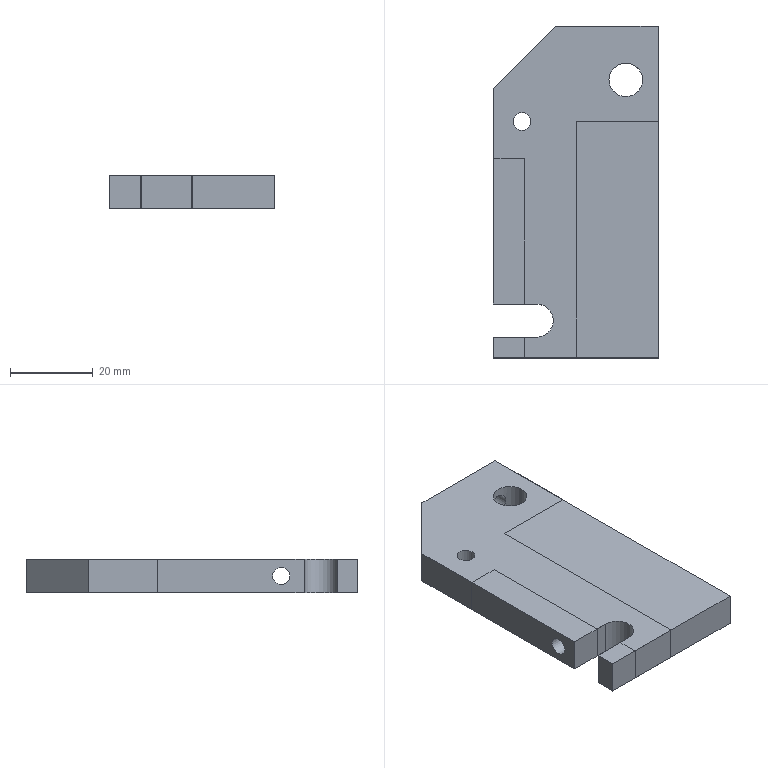Part | 2 solids | 42 faces | box 40 x 80 x 8 mm | volume 34060 mm3 | plane 32 | cylinder 10 | commonest cylinder face diameters 4.2 x4 4.3 x2 8 x2 8.1 x2
STEP:
#1=CARTESIAN_POINT('',(20.,39.8,-8.));
#2=VERTEX_POINT('',#1);
#3=CARTESIAN_POINT('',(19.8,40.,-8.));
#4=VERTEX_POINT('',#3);
#5=CARTESIAN_POINT('',(20.,39.8,-8.));
#6=DIRECTION('',(-0.7071,0.7071,0.));
#7=VECTOR('',#6,1000.);
#8=LINE('',#5,#7);
#9=EDGE_CURVE('',#2,#4,#8,.T.);
#10=ORIENTED_EDGE('',*,*,#9,.T.);
#11=CARTESIAN_POINT('',(19.8,40.,0.));
#12=VERTEX_POINT('',#11);
#13=CARTESIAN_POINT('',(19.8,40.,-8.));
#14=DIRECTION('',(0.,0.,-1.));
#15=VECTOR('',#14,1000.);
#16=LINE('',#13,#15);
#17=EDGE_CURVE('',#12,#4,#16,.T.);
#18=ORIENTED_EDGE('',*,*,#17,.F.);
#19=CARTESIAN_POINT('',(20.,39.8,0.));
#20=VERTEX_POINT('',#19);
#21=CARTESIAN_POINT('',(40.65,19.15,0.));
#22=DIRECTION('',(0.7071,-0.7071,0.));
#23=VECTOR('',#22,1000.);
#24=LINE('',#21,#23);
#25=EDGE_CURVE('',#12,#20,#24,.T.);
#26=ORIENTED_EDGE('',*,*,#25,.T.);
#27=CARTESIAN_POINT('',(20.,39.8,-8.));
#28=DIRECTION('',(0.,0.,1.));
#29=VECTOR('',#28,1000.);
#30=LINE('',#27,#29);
#31=EDGE_CURVE('',#2,#20,#30,.T.);
#32=ORIENTED_EDGE('',*,*,#31,.F.);
#33=EDGE_LOOP('',(#10,#18,#26,#32));
#34=FACE_BOUND('',#33,.T.);
#35=CARTESIAN_POINT('',(20.,39.8,-8.));
#36=DIRECTION('',(-0.7071,-0.7071,0.));
#37=DIRECTION('',(0.,0.,1.));
#38=AXIS2_PLACEMENT_3D('',#35,#36,#37);
#39=PLANE('',#38);
#40=ADVANCED_FACE('',(#34),#39,.F.);
#41=CARTESIAN_POINT('',(-20.,-21.5,-6.1));
#42=VERTEX_POINT('',#41);
#43=CARTESIAN_POINT('',(-20.,-21.5,-4.));
#44=DIRECTION('',(1.,0.,0.));
#45=DIRECTION('',(0.,0.,-1.));
#46=AXIS2_PLACEMENT_3D('',#43,#44,#45);
#47=CIRCLE('',#46,2.1);
#48=EDGE_CURVE('',#42,#42,#47,.F.);
#49=ORIENTED_EDGE('',*,*,#48,.T.);
#50=EDGE_LOOP('',(#49));
#51=FACE_BOUND('',#50,.T.);
#52=CARTESIAN_POINT('',(20.,-21.5,-1.9));
#53=VERTEX_POINT('',#52);
#54=CARTESIAN_POINT('',(20.,-21.5,-4.));
#55=DIRECTION('',(-1.,0.,0.));
#56=DIRECTION('',(0.,0.,1.));
#57=AXIS2_PLACEMENT_3D('',#54,#55,#56);
#58=CIRCLE('',#57,2.1);
#59=EDGE_CURVE('',#53,#53,#58,.F.);
#60=ORIENTED_EDGE('',*,*,#59,.T.);
#61=EDGE_LOOP('',(#60));
#62=FACE_BOUND('',#61,.T.);
#63=CARTESIAN_POINT('',(0.1,-21.5,-4.));
#64=DIRECTION('',(-1.,0.,0.));
#65=DIRECTION('',(0.,0.,1.));
#66=AXIS2_PLACEMENT_3D('',#63,#64,#65);
#67=CYLINDRICAL_SURFACE('',#66,2.1);
#68=ADVANCED_FACE('',(#51,#62),#67,.F.);
#69=CARTESIAN_POINT('',(12.,31.05,-1.9));
#70=VERTEX_POINT('',#69);
#71=CARTESIAN_POINT('',(12.704,31.005,-1.982));
#72=CARTESIAN_POINT('',(12.022,31.078,-1.85));
#73=CARTESIAN_POINT('',(11.33,31.011,-1.971));
#74=CARTESIAN_POINT('',(10.827,30.881,-2.248));
#75=CARTESIAN_POINT('',(10.609,30.808,-2.406));
#76=CARTESIAN_POINT('',(10.332,30.692,-2.717));
#77=CARTESIAN_POINT('',(10.245,30.65,-2.843));
#78=CARTESIAN_POINT('',(10.049,30.552,-3.178));
#79=CARTESIAN_POINT('',(9.934,30.483,-3.561));
#80=CARTESIAN_POINT('',(9.886,30.454,-3.986));
#81=CARTESIAN_POINT('',(9.923,30.477,-4.399));
#82=CARTESIAN_POINT('',(10.032,30.54,-4.747));
#83=CARTESIAN_POINT('',(10.127,30.592,-4.96));
#84=CARTESIAN_POINT('',(10.26,30.657,-5.18));
#85=CARTESIAN_POINT('',(10.309,30.681,-5.25));
#86=CARTESIAN_POINT('',(10.494,30.762,-5.473));
#87=CARTESIAN_POINT('',(10.676,30.828,-5.633));
#88=CARTESIAN_POINT('',(10.855,30.887,-5.768));
#89=CARTESIAN_POINT('',(11.288,31.003,-6.012));
#90=CARTESIAN_POINT('',(11.973,31.078,-6.15));
#91=CARTESIAN_POINT('',(12.659,31.013,-6.034));
#92=CARTESIAN_POINT('',(13.172,30.881,-5.752));
#93=CARTESIAN_POINT('',(13.393,30.807,-5.592));
#94=CARTESIAN_POINT('',(13.668,30.692,-5.283));
#95=CARTESIAN_POINT('',(13.756,30.65,-5.156));
#96=CARTESIAN_POINT('',(13.95,30.552,-4.823));
#97=CARTESIAN_POINT('',(14.067,30.483,-4.439));
#98=CARTESIAN_POINT('',(14.114,30.455,-4.013));
#99=CARTESIAN_POINT('',(14.078,30.477,-3.605));
#100=CARTESIAN_POINT('',(13.969,30.54,-3.254));
#101=CARTESIAN_POINT('',(13.873,30.592,-3.042));
#102=CARTESIAN_POINT('',(13.743,30.656,-2.824));
#103=CARTESIAN_POINT('',(13.691,30.681,-2.751));
#104=CARTESIAN_POINT('',(13.508,30.761,-2.529));
#105=CARTESIAN_POINT('',(13.326,30.828,-2.369));
#106=CARTESIAN_POINT('',(13.148,30.886,-2.235));
#107=CARTESIAN_POINT('',(12.704,31.005,-1.982));
#108=CARTESIAN_POINT('',(12.022,31.078,-1.85));
#109=CARTESIAN_POINT('',(11.33,31.011,-1.971));
#110=B_SPLINE_CURVE_WITH_KNOTS('',3,(#71,#72,#73,#74,#75,#76,#77,#78,#79,#80,#81,#82,#83,#84,#85,#86,#87,#88,#89,#90,#91,#92,#93,#94,#95,#96,#97,#98,#99,#100,#101,#102,#103,#104,#105,#106,#107,#108,#109),.UNSPECIFIED.,.T.,.F.,(1,1,1,1,1,1,1,1,1,1,1,1,1,1,1,1,1,1,1,1,1,1,1,1,1,1,1,1,1,1,1,1,1,1,1,1,1,1,1,1,1,1,1),(-0.111,-0.09539,-0.06414,0.,0.05937,0.09203,0.1234,0.139,0.1546,0.1859,0.2171,0.2484,0.2796,0.3109,0.3265,0.3421,0.3577,0.3734,0.389,0.4046,0.4359,0.4968,0.5592,0.592,0.6234,0.639,0.6546,0.6859,0.7171,0.7484,0.7796,0.8109,0.8265,0.8421,0.8577,0.8734,0.889,0.9046,0.9359,1.,1.059,1.092,1.123),.UNSPECIFIED.);
#111=EDGE_CURVE('',#70,#70,#110,.F.);
#112=ORIENTED_EDGE('',*,*,#111,.F.);
#113=EDGE_LOOP('',(#112));
#114=FACE_BOUND('',#113,.T.);
#115=CARTESIAN_POINT('',(9.9,40.,-4.));
#116=VERTEX_POINT('',#115);
#117=CARTESIAN_POINT('',(12.,40.,-4.));
#118=DIRECTION('',(0.,1.,0.));
#119=DIRECTION('',(-1.,0.,0.));
#120=AXIS2_PLACEMENT_3D('',#117,#118,#119);
#121=CIRCLE('',#120,2.1);
#122=EDGE_CURVE('',#116,#116,#121,.T.);
#123=ORIENTED_EDGE('',*,*,#122,.T.);
#124=EDGE_LOOP('',(#123));
#125=FACE_BOUND('',#124,.T.);
#126=CARTESIAN_POINT('',(12.,27.,-4.));
#127=DIRECTION('',(0.,1.,0.));
#128=DIRECTION('',(0.,0.,1.));
#129=AXIS2_PLACEMENT_3D('',#126,#127,#128);
#130=CYLINDRICAL_SURFACE('',#129,2.1);
#131=ADVANCED_FACE('',(#114,#125),#130,.F.);
#132=CARTESIAN_POINT('',(16.05,27.,0.));
#133=VERTEX_POINT('',#132);
#134=CARTESIAN_POINT('',(12.,27.,0.));
#135=DIRECTION('',(0.,0.,1.));
#136=DIRECTION('',(1.,0.,0.));
#137=AXIS2_PLACEMENT_3D('',#134,#135,#136);
#138=CIRCLE('',#137,4.05);
#139=EDGE_CURVE('',#133,#133,#138,.T.);
#140=ORIENTED_EDGE('',*,*,#139,.F.);
#141=EDGE_LOOP('',(#140));
#142=FACE_BOUND('',#141,.T.);
#143=CARTESIAN_POINT('',(-10.85,17.,0.));
#144=VERTEX_POINT('',#143);
#145=CARTESIAN_POINT('',(-13.,17.,0.));
#146=DIRECTION('',(0.,0.,1.));
#147=DIRECTION('',(1.,0.,0.));
#148=AXIS2_PLACEMENT_3D('',#145,#146,#147);
#149=CIRCLE('',#148,2.15);
#150=EDGE_CURVE('',#144,#144,#149,.T.);
#151=ORIENTED_EDGE('',*,*,#150,.F.);
#152=EDGE_LOOP('',(#151));
#153=FACE_BOUND('',#152,.T.);
#154=CARTESIAN_POINT('',(-9.5,-35.,0.));
#155=VERTEX_POINT('',#154);
#156=CARTESIAN_POINT('',(-20.,-35.,0.));
#157=VERTEX_POINT('',#156);
#158=CARTESIAN_POINT('',(-9.5,-35.,0.));
#159=DIRECTION('',(-1.,0.,0.));
#160=VECTOR('',#159,1000.);
#161=LINE('',#158,#160);
#162=EDGE_CURVE('',#155,#157,#161,.T.);
#163=ORIENTED_EDGE('',*,*,#162,.T.);
#164=CARTESIAN_POINT('',(-20.,-40.,0.));
#165=VERTEX_POINT('',#164);
#166=CARTESIAN_POINT('',(-20.,-31.,0.));
#167=DIRECTION('',(0.,1.,0.));
#168=VECTOR('',#167,1000.);
#169=LINE('',#166,#168);
#170=EDGE_CURVE('',#165,#157,#169,.T.);
#171=ORIENTED_EDGE('',*,*,#170,.F.);
#172=CARTESIAN_POINT('',(20.,-40.,0.));
#173=VERTEX_POINT('',#172);
#174=CARTESIAN_POINT('',(0.,-40.,0.));
#175=DIRECTION('',(-1.,0.,0.));
#176=VECTOR('',#175,1000.);
#177=LINE('',#174,#176);
#178=EDGE_CURVE('',#173,#165,#177,.T.);
#179=ORIENTED_EDGE('',*,*,#178,.F.);
#180=CARTESIAN_POINT('',(20.,40.,0.));
#181=DIRECTION('',(0.,-1.,0.));
#182=VECTOR('',#181,1000.);
#183=LINE('',#180,#182);
#184=EDGE_CURVE('',#173,#20,#183,.F.);
#185=ORIENTED_EDGE('',*,*,#184,.T.);
#186=ORIENTED_EDGE('',*,*,#25,.F.);
#187=CARTESIAN_POINT('',(-5.,40.,0.));
#188=VERTEX_POINT('',#187);
#189=CARTESIAN_POINT('',(-5.,40.,0.));
#190=DIRECTION('',(1.,0.,0.));
#191=VECTOR('',#190,1000.);
#192=LINE('',#189,#191);
#193=EDGE_CURVE('',#188,#12,#192,.T.);
#194=ORIENTED_EDGE('',*,*,#193,.F.);
#195=CARTESIAN_POINT('',(-20.,25.,0.));
#196=VERTEX_POINT('',#195);
#197=CARTESIAN_POINT('',(-20.,25.,0.));
#198=DIRECTION('',(0.7071,0.7071,0.));
#199=VECTOR('',#198,1000.);
#200=LINE('',#197,#199);
#201=EDGE_CURVE('',#196,#188,#200,.T.);
#202=ORIENTED_EDGE('',*,*,#201,.F.);
#203=CARTESIAN_POINT('',(-20.,-27.,0.));
#204=VERTEX_POINT('',#203);
#205=CARTESIAN_POINT('',(-20.,-31.,0.));
#206=DIRECTION('',(0.,1.,0.));
#207=VECTOR('',#206,1000.);
#208=LINE('',#205,#207);
#209=EDGE_CURVE('',#204,#196,#208,.T.);
#210=ORIENTED_EDGE('',*,*,#209,.F.);
#211=CARTESIAN_POINT('',(-9.5,-27.,0.));
#212=VERTEX_POINT('',#211);
#213=CARTESIAN_POINT('',(-9.5,-27.,0.));
#214=DIRECTION('',(-1.,0.,0.));
#215=VECTOR('',#214,1000.);
#216=LINE('',#213,#215);
#217=EDGE_CURVE('',#212,#204,#216,.T.);
#218=ORIENTED_EDGE('',*,*,#217,.F.);
#219=CARTESIAN_POINT('',(-9.5,-31.,0.));
#220=DIRECTION('',(0.,0.,1.));
#221=DIRECTION('',(1.,0.,0.));
#222=AXIS2_PLACEMENT_3D('',#219,#220,#221);
#223=CIRCLE('',#222,4.);
#224=EDGE_CURVE('',#155,#212,#223,.T.);
#225=ORIENTED_EDGE('',*,*,#224,.F.);
#226=EDGE_LOOP('',(#163,#171,#179,#185,#186,#194,#202,#210,#218,#225));
#227=FACE_BOUND('',#226,.T.);
#228=CARTESIAN_POINT('',(-9.5,-31.,0.));
#229=DIRECTION('',(0.,0.,1.));
#230=DIRECTION('',(1.,0.,0.));
#231=AXIS2_PLACEMENT_3D('',#228,#229,#230);
#232=PLANE('',#231);
#233=ADVANCED_FACE('',(#142,#153,#227),#232,.T.);
#234=CARTESIAN_POINT('',(16.05,27.,-8.));
#235=VERTEX_POINT('',#234);
#236=CARTESIAN_POINT('',(12.,27.,-8.));
#237=DIRECTION('',(0.,0.,1.));
#238=DIRECTION('',(1.,0.,0.));
#239=AXIS2_PLACEMENT_3D('',#236,#237,#238);
#240=CIRCLE('',#239,4.05);
#241=EDGE_CURVE('',#235,#235,#240,.T.);
#242=ORIENTED_EDGE('',*,*,#241,.T.);
#243=EDGE_LOOP('',(#242));
#244=FACE_BOUND('',#243,.T.);
#245=CARTESIAN_POINT('',(-10.85,17.,-8.));
#246=VERTEX_POINT('',#245);
#247=CARTESIAN_POINT('',(-13.,17.,-8.));
#248=DIRECTION('',(0.,0.,1.));
#249=DIRECTION('',(1.,0.,0.));
#250=AXIS2_PLACEMENT_3D('',#247,#248,#249);
#251=CIRCLE('',#250,2.15);
#252=EDGE_CURVE('',#246,#246,#251,.T.);
#253=ORIENTED_EDGE('',*,*,#252,.T.);
#254=EDGE_LOOP('',(#253));
#255=FACE_BOUND('',#254,.T.);
#256=CARTESIAN_POINT('',(-20.,-40.,-8.));
#257=VERTEX_POINT('',#256);
#258=CARTESIAN_POINT('',(-20.,-35.,-8.));
#259=VERTEX_POINT('',#258);
#260=CARTESIAN_POINT('',(-20.,-31.,-8.));
#261=DIRECTION('',(0.,1.,0.));
#262=VECTOR('',#261,1000.);
#263=LINE('',#260,#262);
#264=EDGE_CURVE('',#257,#259,#263,.T.);
#265=ORIENTED_EDGE('',*,*,#264,.T.);
#266=CARTESIAN_POINT('',(-9.5,-35.,-8.));
#267=VERTEX_POINT('',#266);
#268=CARTESIAN_POINT('',(-9.5,-35.,-8.));
#269=DIRECTION('',(-1.,0.,0.));
#270=VECTOR('',#269,1000.);
#271=LINE('',#268,#270);
#272=EDGE_CURVE('',#267,#259,#271,.T.);
#273=ORIENTED_EDGE('',*,*,#272,.F.);
#274=CARTESIAN_POINT('',(-9.5,-27.,-8.));
#275=VERTEX_POINT('',#274);
#276=CARTESIAN_POINT('',(-9.5,-31.,-8.));
#277=DIRECTION('',(0.,0.,1.));
#278=DIRECTION('',(1.,0.,0.));
#279=AXIS2_PLACEMENT_3D('',#276,#277,#278);
#280=CIRCLE('',#279,4.);
#281=EDGE_CURVE('',#267,#275,#280,.T.);
#282=ORIENTED_EDGE('',*,*,#281,.T.);
#283=CARTESIAN_POINT('',(-20.,-27.,-8.));
#284=VERTEX_POINT('',#283);
#285=CARTESIAN_POINT('',(-9.5,-27.,-8.));
#286=DIRECTION('',(-1.,0.,0.));
#287=VECTOR('',#286,1000.);
#288=LINE('',#285,#287);
#289=EDGE_CURVE('',#275,#284,#288,.T.);
#290=ORIENTED_EDGE('',*,*,#289,.T.);
#291=CARTESIAN_POINT('',(-20.,25.,-8.));
#292=VERTEX_POINT('',#291);
#293=CARTESIAN_POINT('',(-20.,-31.,-8.));
#294=DIRECTION('',(0.,1.,0.));
#295=VECTOR('',#294,1000.);
#296=LINE('',#293,#295);
#297=EDGE_CURVE('',#284,#292,#296,.T.);
#298=ORIENTED_EDGE('',*,*,#297,.T.);
#299=CARTESIAN_POINT('',(-5.,40.,-8.));
#300=VERTEX_POINT('',#299);
#301=CARTESIAN_POINT('',(-20.,25.,-8.));
#302=DIRECTION('',(0.7071,0.7071,0.));
#303=VECTOR('',#302,1000.);
#304=LINE('',#301,#303);
#305=EDGE_CURVE('',#292,#300,#304,.T.);
#306=ORIENTED_EDGE('',*,*,#305,.T.);
#307=CARTESIAN_POINT('',(-5.,40.,-8.));
#308=DIRECTION('',(1.,0.,0.));
#309=VECTOR('',#308,1000.);
#310=LINE('',#307,#309);
#311=EDGE_CURVE('',#300,#4,#310,.T.);
#312=ORIENTED_EDGE('',*,*,#311,.T.);
#313=ORIENTED_EDGE('',*,*,#9,.F.);
#314=CARTESIAN_POINT('',(20.,-40.,-8.));
#315=VERTEX_POINT('',#314);
#316=CARTESIAN_POINT('',(20.,40.,-8.));
#317=DIRECTION('',(0.,-1.,0.));
#318=VECTOR('',#317,1000.);
#319=LINE('',#316,#318);
#320=EDGE_CURVE('',#315,#2,#319,.F.);
#321=ORIENTED_EDGE('',*,*,#320,.F.);
#322=CARTESIAN_POINT('',(0.,-40.,-8.));
#323=DIRECTION('',(-1.,0.,0.));
#324=VECTOR('',#323,1000.);
#325=LINE('',#322,#324);
#326=EDGE_CURVE('',#315,#257,#325,.T.);
#327=ORIENTED_EDGE('',*,*,#326,.T.);
#328=EDGE_LOOP('',(#265,#273,#282,#290,#298,#306,#312,#313,#321,#327));
#329=FACE_BOUND('',#328,.T.);
#330=CARTESIAN_POINT('',(-9.5,-31.,-8.));
#331=DIRECTION('',(0.,0.,1.));
#332=DIRECTION('',(1.,0.,0.));
#333=AXIS2_PLACEMENT_3D('',#330,#331,#332);
#334=PLANE('',#333);
#335=ADVANCED_FACE('',(#244,#255,#329),#334,.F.);
#336=ORIENTED_EDGE('',*,*,#150,.T.);
#337=EDGE_LOOP('',(#336));
#338=FACE_BOUND('',#337,.T.);
#339=ORIENTED_EDGE('',*,*,#252,.F.);
#340=EDGE_LOOP('',(#339));
#341=FACE_BOUND('',#340,.T.);
#342=CARTESIAN_POINT('',(-13.,17.,-8.));
#343=DIRECTION('',(0.,0.,1.));
#344=DIRECTION('',(1.,0.,0.));
#345=AXIS2_PLACEMENT_3D('',#342,#343,#344);
#346=CYLINDRICAL_SURFACE('',#345,2.15);
#347=ADVANCED_FACE('',(#338,#341),#346,.F.);
#348=ORIENTED_EDGE('',*,*,#111,.T.);
#349=EDGE_LOOP('',(#348));
#350=FACE_BOUND('',#349,.T.);
#351=ORIENTED_EDGE('',*,*,#139,.T.);
#352=EDGE_LOOP('',(#351));
#353=FACE_BOUND('',#352,.T.);
#354=ORIENTED_EDGE('',*,*,#241,.F.);
#355=EDGE_LOOP('',(#354));
#356=FACE_BOUND('',#355,.T.);
#357=CARTESIAN_POINT('',(12.,27.,-8.));
#358=DIRECTION('',(0.,0.,1.));
#359=DIRECTION('',(1.,0.,0.));
#360=AXIS2_PLACEMENT_3D('',#357,#358,#359);
#361=CYLINDRICAL_SURFACE('',#360,4.05);
#362=ADVANCED_FACE('',(#350,#353,#356),#361,.F.);
#363=ORIENTED_EDGE('',*,*,#320,.T.);
#364=ORIENTED_EDGE('',*,*,#31,.T.);
#365=ORIENTED_EDGE('',*,*,#184,.F.);
#366=CARTESIAN_POINT('',(20.,-40.,-8.));
#367=DIRECTION('',(0.,0.,1.));
#368=VECTOR('',#367,1000.);
#369=LINE('',#366,#368);
#370=EDGE_CURVE('',#173,#315,#369,.F.);
#371=ORIENTED_EDGE('',*,*,#370,.T.);
#372=EDGE_LOOP('',(#363,#364,#365,#371));
#373=FACE_BOUND('',#372,.T.);
#374=ORIENTED_EDGE('',*,*,#59,.F.);
#375=EDGE_LOOP('',(#374));
#376=FACE_BOUND('',#375,.T.);
#377=CARTESIAN_POINT('',(20.,40.,-8.));
#378=DIRECTION('',(-1.,0.,0.));
#379=DIRECTION('',(0.,0.,1.));
#380=AXIS2_PLACEMENT_3D('',#377,#378,#379);
#381=PLANE('',#380);
#382=ADVANCED_FACE('',(#373,#376),#381,.F.);
#383=ORIENTED_EDGE('',*,*,#122,.F.);
#384=EDGE_LOOP('',(#383));
#385=FACE_BOUND('',#384,.T.);
#386=ORIENTED_EDGE('',*,*,#193,.T.);
#387=ORIENTED_EDGE('',*,*,#17,.T.);
#388=ORIENTED_EDGE('',*,*,#311,.F.);
#389=CARTESIAN_POINT('',(-5.,40.,-8.));
#390=DIRECTION('',(0.,0.,1.));
#391=VECTOR('',#390,1000.);
#392=LINE('',#389,#391);
#393=EDGE_CURVE('',#300,#188,#392,.T.);
#394=ORIENTED_EDGE('',*,*,#393,.T.);
#395=EDGE_LOOP('',(#386,#387,#388,#394));
#396=FACE_BOUND('',#395,.T.);
#397=CARTESIAN_POINT('',(-5.,40.,-8.));
#398=DIRECTION('',(0.,-1.,0.));
#399=DIRECTION('',(0.,0.,-1.));
#400=AXIS2_PLACEMENT_3D('',#397,#398,#399);
#401=PLANE('',#400);
#402=ADVANCED_FACE('',(#385,#396),#401,.F.);
#403=ORIENTED_EDGE('',*,*,#201,.T.);
#404=ORIENTED_EDGE('',*,*,#393,.F.);
#405=ORIENTED_EDGE('',*,*,#305,.F.);
#406=CARTESIAN_POINT('',(-20.,25.,-8.));
#407=DIRECTION('',(0.,0.,1.));
#408=VECTOR('',#407,1000.);
#409=LINE('',#406,#408);
#410=EDGE_CURVE('',#292,#196,#409,.T.);
#411=ORIENTED_EDGE('',*,*,#410,.T.);
#412=EDGE_LOOP('',(#403,#404,#405,#411));
#413=FACE_BOUND('',#412,.T.);
#414=CARTESIAN_POINT('',(-20.,25.,-8.));
#415=DIRECTION('',(0.7071,-0.7071,0.));
#416=DIRECTION('',(0.7071,0.7071,0.));
#417=AXIS2_PLACEMENT_3D('',#414,#415,#416);
#418=PLANE('',#417);
#419=ADVANCED_FACE('',(#413),#418,.F.);
#420=ORIENTED_EDGE('',*,*,#48,.F.);
#421=EDGE_LOOP('',(#420));
#422=FACE_BOUND('',#421,.T.);
#423=ORIENTED_EDGE('',*,*,#297,.F.);
#424=CARTESIAN_POINT('',(-20.,-27.,-8.));
#425=DIRECTION('',(0.,0.,1.));
#426=VECTOR('',#425,1000.);
#427=LINE('',#424,#426);
#428=EDGE_CURVE('',#204,#284,#427,.F.);
#429=ORIENTED_EDGE('',*,*,#428,.F.);
#430=ORIENTED_EDGE('',*,*,#209,.T.);
#431=ORIENTED_EDGE('',*,*,#410,.F.);
#432=EDGE_LOOP('',(#423,#429,#430,#431));
#433=FACE_BOUND('',#432,.T.);
#434=CARTESIAN_POINT('',(-20.,8.,-8.));
#435=DIRECTION('',(1.,0.,0.));
#436=DIRECTION('',(0.,0.,-1.));
#437=AXIS2_PLACEMENT_3D('',#434,#435,#436);
#438=PLANE('',#437);
#439=ADVANCED_FACE('',(#422,#433),#438,.F.);
#440=ORIENTED_EDGE('',*,*,#217,.T.);
#441=ORIENTED_EDGE('',*,*,#428,.T.);
#442=ORIENTED_EDGE('',*,*,#289,.F.);
#443=CARTESIAN_POINT('',(-9.5,-27.,-8.));
#444=DIRECTION('',(0.,0.,1.));
#445=VECTOR('',#444,1000.);
#446=LINE('',#443,#445);
#447=EDGE_CURVE('',#275,#212,#446,.T.);
#448=ORIENTED_EDGE('',*,*,#447,.T.);
#449=EDGE_LOOP('',(#440,#441,#442,#448));
#450=FACE_BOUND('',#449,.T.);
#451=CARTESIAN_POINT('',(-9.5,-27.,-8.));
#452=DIRECTION('',(0.,1.,0.));
#453=DIRECTION('',(0.,0.,1.));
#454=AXIS2_PLACEMENT_3D('',#451,#452,#453);
#455=PLANE('',#454);
#456=ADVANCED_FACE('',(#450),#455,.F.);
#457=ORIENTED_EDGE('',*,*,#224,.T.);
#458=ORIENTED_EDGE('',*,*,#447,.F.);
#459=ORIENTED_EDGE('',*,*,#281,.F.);
#460=CARTESIAN_POINT('',(-9.5,-35.,-8.));
#461=DIRECTION('',(0.,0.,1.));
#462=VECTOR('',#461,1000.);
#463=LINE('',#460,#462);
#464=EDGE_CURVE('',#267,#155,#463,.T.);
#465=ORIENTED_EDGE('',*,*,#464,.T.);
#466=EDGE_LOOP('',(#457,#458,#459,#465));
#467=FACE_BOUND('',#466,.T.);
#468=CARTESIAN_POINT('',(-9.5,-31.,-8.));
#469=DIRECTION('',(0.,0.,1.));
#470=DIRECTION('',(1.,0.,0.));
#471=AXIS2_PLACEMENT_3D('',#468,#469,#470);
#472=CYLINDRICAL_SURFACE('',#471,4.);
#473=ADVANCED_FACE('',(#467),#472,.F.);
#474=ORIENTED_EDGE('',*,*,#272,.T.);
#475=CARTESIAN_POINT('',(-20.,-35.,-8.));
#476=DIRECTION('',(0.,0.,-1.));
#477=VECTOR('',#476,1000.);
#478=LINE('',#475,#477);
#479=EDGE_CURVE('',#157,#259,#478,.T.);
#480=ORIENTED_EDGE('',*,*,#479,.F.);
#481=ORIENTED_EDGE('',*,*,#162,.F.);
#482=ORIENTED_EDGE('',*,*,#464,.F.);
#483=EDGE_LOOP('',(#474,#480,#481,#482));
#484=FACE_BOUND('',#483,.T.);
#485=CARTESIAN_POINT('',(-9.5,-35.,-8.));
#486=DIRECTION('',(0.,1.,0.));
#487=DIRECTION('',(0.,0.,1.));
#488=AXIS2_PLACEMENT_3D('',#485,#486,#487);
#489=PLANE('',#488);
#490=ADVANCED_FACE('',(#484),#489,.T.);
#491=ORIENTED_EDGE('',*,*,#170,.T.);
#492=ORIENTED_EDGE('',*,*,#479,.T.);
#493=ORIENTED_EDGE('',*,*,#264,.F.);
#494=CARTESIAN_POINT('',(-20.,-40.,-8.));
#495=DIRECTION('',(0.,0.,-1.));
#496=VECTOR('',#495,1000.);
#497=LINE('',#494,#496);
#498=EDGE_CURVE('',#165,#257,#497,.T.);
#499=ORIENTED_EDGE('',*,*,#498,.F.);
#500=EDGE_LOOP('',(#491,#492,#493,#499));
#501=FACE_BOUND('',#500,.T.);
#502=CARTESIAN_POINT('',(-20.,8.,-8.));
#503=DIRECTION('',(1.,0.,0.));
#504=DIRECTION('',(0.,0.,-1.));
#505=AXIS2_PLACEMENT_3D('',#502,#503,#504);
#506=PLANE('',#505);
#507=ADVANCED_FACE('',(#501),#506,.F.);
#508=ORIENTED_EDGE('',*,*,#178,.T.);
#509=ORIENTED_EDGE('',*,*,#498,.T.);
#510=ORIENTED_EDGE('',*,*,#326,.F.);
#511=ORIENTED_EDGE('',*,*,#370,.F.);
#512=EDGE_LOOP('',(#508,#509,#510,#511));
#513=FACE_BOUND('',#512,.T.);
#514=CARTESIAN_POINT('',(0.,-40.,-8.));
#515=DIRECTION('',(0.,1.,0.));
#516=DIRECTION('',(0.,0.,1.));
#517=AXIS2_PLACEMENT_3D('',#514,#515,#516);
#518=PLANE('',#517);
#519=ADVANCED_FACE('',(#513),#518,.F.);
#520=CLOSED_SHELL('',(#40,#68,#131,#233,#335,#347,#362,#382,#402,#419,#439,#456,#473,#490,#507,#519));
#521=MANIFOLD_SOLID_BREP('',#520);
#522=CARTESIAN_POINT('',(19.8,17.,-8.));
#523=VERTEX_POINT('',#522);
#524=CARTESIAN_POINT('',(20.,17.2,-8.));
#525=VERTEX_POINT('',#524);
#526=CARTESIAN_POINT('',(19.8,17.,-8.));
#527=DIRECTION('',(0.7071,0.7071,0.));
#528=VECTOR('',#527,1000.);
#529=LINE('',#526,#528);
#530=EDGE_CURVE('',#523,#525,#529,.T.);
#531=ORIENTED_EDGE('',*,*,#530,.T.);
#532=CARTESIAN_POINT('',(20.,17.2,0.));
#533=VERTEX_POINT('',#532);
#534=CARTESIAN_POINT('',(20.,17.2,-8.));
#535=DIRECTION('',(0.,0.,-1.));
#536=VECTOR('',#535,1000.);
#537=LINE('',#534,#536);
#538=EDGE_CURVE('',#533,#525,#537,.T.);
#539=ORIENTED_EDGE('',*,*,#538,.F.);
#540=CARTESIAN_POINT('',(19.8,17.,0.));
#541=VERTEX_POINT('',#540);
#542=CARTESIAN_POINT('',(-18.85,-21.65,0.));
#543=DIRECTION('',(-0.7071,-0.7071,0.));
#544=VECTOR('',#543,1000.);
#545=LINE('',#542,#544);
#546=EDGE_CURVE('',#533,#541,#545,.T.);
#547=ORIENTED_EDGE('',*,*,#546,.T.);
#548=CARTESIAN_POINT('',(19.8,17.,-8.));
#549=DIRECTION('',(0.,0.,1.));
#550=VECTOR('',#549,1000.);
#551=LINE('',#548,#550);
#552=EDGE_CURVE('',#523,#541,#551,.T.);
#553=ORIENTED_EDGE('',*,*,#552,.F.);
#554=EDGE_LOOP('',(#531,#539,#547,#553));
#555=FACE_BOUND('',#554,.T.);
#556=CARTESIAN_POINT('',(19.8,17.,-8.));
#557=DIRECTION('',(-0.7071,0.7071,0.));
#558=DIRECTION('',(0.,0.,1.));
#559=AXIS2_PLACEMENT_3D('',#556,#557,#558);
#560=PLANE('',#559);
#561=ADVANCED_FACE('',(#555),#560,.F.);
#562=CARTESIAN_POINT('',(20.,39.8,-8.));
#563=VERTEX_POINT('',#562);
#564=CARTESIAN_POINT('',(19.8,40.,-8.));
#565=VERTEX_POINT('',#564);
#566=CARTESIAN_POINT('',(20.,39.8,-8.));
#567=DIRECTION('',(-0.7071,0.7071,0.));
#568=VECTOR('',#567,1000.);
#569=LINE('',#566,#568);
#570=EDGE_CURVE('',#563,#565,#569,.T.);
#571=ORIENTED_EDGE('',*,*,#570,.T.);
#572=CARTESIAN_POINT('',(19.8,40.,0.));
#573=VERTEX_POINT('',#572);
#574=CARTESIAN_POINT('',(19.8,40.,-8.));
#575=DIRECTION('',(0.,0.,-1.));
#576=VECTOR('',#575,1000.);
#577=LINE('',#574,#576);
#578=EDGE_CURVE('',#573,#565,#577,.T.);
#579=ORIENTED_EDGE('',*,*,#578,.F.);
#580=CARTESIAN_POINT('',(20.,39.8,0.));
#581=VERTEX_POINT('',#580);
#582=CARTESIAN_POINT('',(40.65,19.15,0.));
#583=DIRECTION('',(0.7071,-0.7071,0.));
#584=VECTOR('',#583,1000.);
#585=LINE('',#582,#584);
#586=EDGE_CURVE('',#573,#581,#585,.T.);
#587=ORIENTED_EDGE('',*,*,#586,.T.);
#588=CARTESIAN_POINT('',(20.,39.8,-8.));
#589=DIRECTION('',(0.,0.,1.));
#590=VECTOR('',#589,1000.);
#591=LINE('',#588,#590);
#592=EDGE_CURVE('',#563,#581,#591,.T.);
#593=ORIENTED_EDGE('',*,*,#592,.F.);
#594=EDGE_LOOP('',(#571,#579,#587,#593));
#595=FACE_BOUND('',#594,.T.);
#596=CARTESIAN_POINT('',(20.,39.8,-8.));
#597=DIRECTION('',(-0.7071,-0.7071,0.));
#598=DIRECTION('',(0.,0.,1.));
#599=AXIS2_PLACEMENT_3D('',#596,#597,#598);
#600=PLANE('',#599);
#601=ADVANCED_FACE('',(#595),#600,.F.);
#602=CARTESIAN_POINT('',(0.,-39.8,-8.));
#603=VERTEX_POINT('',#602);
#604=CARTESIAN_POINT('',(-0.2,-40.,-8.));
#605=VERTEX_POINT('',#604);
#606=CARTESIAN_POINT('',(-0.2,-40.,-8.));
#607=DIRECTION('',(-0.7071,-0.7071,0.));
#608=VECTOR('',#607,1000.);
#609=LINE('',#606,#608);
#610=EDGE_CURVE('',#603,#605,#609,.T.);
#611=ORIENTED_EDGE('',*,*,#610,.F.);
#612=CARTESIAN_POINT('',(0.,-39.8,0.));
#613=VERTEX_POINT('',#612);
#614=CARTESIAN_POINT('',(0.,-39.8,-8.));
#615=DIRECTION('',(0.,0.,-1.));
#616=VECTOR('',#615,1000.);
#617=LINE('',#614,#616);
#618=EDGE_CURVE('',#613,#603,#617,.T.);
#619=ORIENTED_EDGE('',*,*,#618,.F.);
#620=CARTESIAN_POINT('',(-0.2,-40.,0.));
#621=VERTEX_POINT('',#620);
#622=CARTESIAN_POINT('',(-0.35,-40.15,0.));
#623=DIRECTION('',(0.7071,0.7071,0.));
#624=VECTOR('',#623,1000.);
#625=LINE('',#622,#624);
#626=EDGE_CURVE('',#621,#613,#625,.T.);
#627=ORIENTED_EDGE('',*,*,#626,.F.);
#628=CARTESIAN_POINT('',(-0.2,-40.,0.));
#629=DIRECTION('',(0.,0.,1.));
#630=VECTOR('',#629,1000.);
#631=LINE('',#628,#630);
#632=EDGE_CURVE('',#605,#621,#631,.T.);
#633=ORIENTED_EDGE('',*,*,#632,.F.);
#634=EDGE_LOOP('',(#611,#619,#627,#633));
#635=FACE_BOUND('',#634,.T.);
#636=CARTESIAN_POINT('',(-0.2,-40.,-8.));
#637=DIRECTION('',(0.7071,-0.7071,0.));
#638=DIRECTION('',(0.,0.,-1.));
#639=AXIS2_PLACEMENT_3D('',#636,#637,#638);
#640=PLANE('',#639);
#641=ADVANCED_FACE('',(#635),#640,.T.);
#642=CARTESIAN_POINT('',(-12.4,-39.8,-8.));
#643=VERTEX_POINT('',#642);
#644=CARTESIAN_POINT('',(-12.2,-40.,-8.));
#645=VERTEX_POINT('',#644);
#646=CARTESIAN_POINT('',(-12.4,-39.8,-8.));
#647=DIRECTION('',(0.7071,-0.7071,0.));
#648=VECTOR('',#647,1000.);
#649=LINE('',#646,#648);
#650=EDGE_CURVE('',#643,#645,#649,.T.);
#651=ORIENTED_EDGE('',*,*,#650,.T.);
#652=CARTESIAN_POINT('',(-12.2,-40.,0.));
#653=VERTEX_POINT('',#652);
#654=CARTESIAN_POINT('',(-12.2,-40.,-8.));
#655=DIRECTION('',(0.,0.,-1.));
#656=VECTOR('',#655,1000.);
#657=LINE('',#654,#656);
#658=EDGE_CURVE('',#653,#645,#657,.T.);
#659=ORIENTED_EDGE('',*,*,#658,.F.);
#660=CARTESIAN_POINT('',(-12.4,-39.8,0.));
#661=VERTEX_POINT('',#660);
#662=CARTESIAN_POINT('',(-15.35,-36.85,0.));
#663=DIRECTION('',(-0.7071,0.7071,0.));
#664=VECTOR('',#663,1000.);
#665=LINE('',#662,#664);
#666=EDGE_CURVE('',#653,#661,#665,.T.);
#667=ORIENTED_EDGE('',*,*,#666,.T.);
#668=CARTESIAN_POINT('',(-12.4,-39.8,-8.));
#669=DIRECTION('',(0.,0.,1.));
#670=VECTOR('',#669,1000.);
#671=LINE('',#668,#670);
#672=EDGE_CURVE('',#643,#661,#671,.T.);
#673=ORIENTED_EDGE('',*,*,#672,.F.);
#674=EDGE_LOOP('',(#651,#659,#667,#673));
#675=FACE_BOUND('',#674,.T.);
#676=CARTESIAN_POINT('',(-12.4,-39.8,-8.));
#677=DIRECTION('',(0.7071,0.7071,0.));
#678=DIRECTION('',(0.,0.,1.));
#679=AXIS2_PLACEMENT_3D('',#676,#677,#678);
#680=PLANE('',#679);
#681=ADVANCED_FACE('',(#675),#680,.F.);
#682=CARTESIAN_POINT('',(-12.2,-27.,-8.));
#683=VERTEX_POINT('',#682);
#684=CARTESIAN_POINT('',(-12.4,-26.8,-8.));
#685=VERTEX_POINT('',#684);
#686=CARTESIAN_POINT('',(-12.4,-26.8,-8.));
#687=DIRECTION('',(-0.7071,0.7071,0.));
#688=VECTOR('',#687,1000.);
#689=LINE('',#686,#688);
#690=EDGE_CURVE('',#683,#685,#689,.T.);
#691=ORIENTED_EDGE('',*,*,#690,.F.);
#692=CARTESIAN_POINT('',(-12.2,-27.,0.));
#693=VERTEX_POINT('',#692);
#694=CARTESIAN_POINT('',(-12.2,-27.,-8.));
#695=DIRECTION('',(0.,0.,-1.));
#696=VECTOR('',#695,1000.);
#697=LINE('',#694,#696);
#698=EDGE_CURVE('',#693,#683,#697,.T.);
#699=ORIENTED_EDGE('',*,*,#698,.F.);
#700=CARTESIAN_POINT('',(-12.4,-26.8,0.));
#701=VERTEX_POINT('',#700);
#702=CARTESIAN_POINT('',(-8.85,-30.35,0.));
#703=DIRECTION('',(0.7071,-0.7071,0.));
#704=VECTOR('',#703,1000.);
#705=LINE('',#702,#704);
#706=EDGE_CURVE('',#701,#693,#705,.T.);
#707=ORIENTED_EDGE('',*,*,#706,.F.);
#708=CARTESIAN_POINT('',(-12.4,-26.8,0.));
#709=DIRECTION('',(0.,0.,1.));
#710=VECTOR('',#709,1000.);
#711=LINE('',#708,#710);
#712=EDGE_CURVE('',#685,#701,#711,.T.);
#713=ORIENTED_EDGE('',*,*,#712,.F.);
#714=EDGE_LOOP('',(#691,#699,#707,#713));
#715=FACE_BOUND('',#714,.T.);
#716=CARTESIAN_POINT('',(-12.4,-26.8,-8.));
#717=DIRECTION('',(-0.7071,-0.7071,0.));
#718=DIRECTION('',(0.,0.,-1.));
#719=AXIS2_PLACEMENT_3D('',#716,#717,#718);
#720=PLANE('',#719);
#721=ADVANCED_FACE('',(#715),#720,.T.);
#722=CARTESIAN_POINT('',(-20.,8.2,-8.));
#723=VERTEX_POINT('',#722);
#724=CARTESIAN_POINT('',(-19.8,8.,-8.));
#725=VERTEX_POINT('',#724);
#726=CARTESIAN_POINT('',(-20.,8.2,-8.));
#727=DIRECTION('',(0.7071,-0.7071,0.));
#728=VECTOR('',#727,1000.);
#729=LINE('',#726,#728);
#730=EDGE_CURVE('',#723,#725,#729,.T.);
#731=ORIENTED_EDGE('',*,*,#730,.T.);
#732=CARTESIAN_POINT('',(-19.8,8.,0.));
#733=VERTEX_POINT('',#732);
#734=CARTESIAN_POINT('',(-19.8,8.,-8.));
#735=DIRECTION('',(0.,0.,-1.));
#736=VECTOR('',#735,1000.);
#737=LINE('',#734,#736);
#738=EDGE_CURVE('',#733,#725,#737,.T.);
#739=ORIENTED_EDGE('',*,*,#738,.F.);
#740=CARTESIAN_POINT('',(-20.,8.2,0.));
#741=VERTEX_POINT('',#740);
#742=CARTESIAN_POINT('',(4.85,-16.65,0.));
#743=DIRECTION('',(-0.7071,0.7071,0.));
#744=VECTOR('',#743,1000.);
#745=LINE('',#742,#744);
#746=EDGE_CURVE('',#733,#741,#745,.T.);
#747=ORIENTED_EDGE('',*,*,#746,.T.);
#748=CARTESIAN_POINT('',(-20.,8.2,-8.));
#749=DIRECTION('',(0.,0.,1.));
#750=VECTOR('',#749,1000.);
#751=LINE('',#748,#750);
#752=EDGE_CURVE('',#723,#741,#751,.T.);
#753=ORIENTED_EDGE('',*,*,#752,.F.);
#754=EDGE_LOOP('',(#731,#739,#747,#753));
#755=FACE_BOUND('',#754,.T.);
#756=CARTESIAN_POINT('',(-20.,8.2,-8.));
#757=DIRECTION('',(0.7071,0.7071,0.));
#758=DIRECTION('',(0.,0.,1.));
#759=AXIS2_PLACEMENT_3D('',#756,#757,#758);
#760=PLANE('',#759);
#761=ADVANCED_FACE('',(#755),#760,.F.);
#762=CARTESIAN_POINT('',(-12.4,-35.2,-8.));
#763=VERTEX_POINT('',#762);
#764=CARTESIAN_POINT('',(-12.2,-35.,-8.));
#765=VERTEX_POINT('',#764);
#766=CARTESIAN_POINT('',(-12.2,-35.,-8.));
#767=DIRECTION('',(0.7071,0.7071,0.));
#768=VECTOR('',#767,1000.);
#769=LINE('',#766,#768);
#770=EDGE_CURVE('',#763,#765,#769,.T.);
#771=ORIENTED_EDGE('',*,*,#770,.F.);
#772=CARTESIAN_POINT('',(-12.4,-35.2,0.));
#773=VERTEX_POINT('',#772);
#774=CARTESIAN_POINT('',(-12.4,-35.2,-8.));
#775=DIRECTION('',(0.,0.,-1.));
#776=VECTOR('',#775,1000.);
#777=LINE('',#774,#776);
#778=EDGE_CURVE('',#773,#763,#777,.T.);
#779=ORIENTED_EDGE('',*,*,#778,.F.);
#780=CARTESIAN_POINT('',(-12.2,-35.,0.));
#781=VERTEX_POINT('',#780);
#782=CARTESIAN_POINT('',(-8.85,-31.65,0.));
#783=DIRECTION('',(-0.7071,-0.7071,0.));
#784=VECTOR('',#783,1000.);
#785=LINE('',#782,#784);
#786=EDGE_CURVE('',#781,#773,#785,.T.);
#787=ORIENTED_EDGE('',*,*,#786,.F.);
#788=CARTESIAN_POINT('',(-12.2,-35.,0.));
#789=DIRECTION('',(0.,0.,1.));
#790=VECTOR('',#789,1000.);
#791=LINE('',#788,#790);
#792=EDGE_CURVE('',#765,#781,#791,.T.);
#793=ORIENTED_EDGE('',*,*,#792,.F.);
#794=EDGE_LOOP('',(#771,#779,#787,#793));
#795=FACE_BOUND('',#794,.T.);
#796=CARTESIAN_POINT('',(-12.2,-35.,-8.));
#797=DIRECTION('',(-0.7071,0.7071,0.));
#798=DIRECTION('',(0.,0.,-1.));
#799=AXIS2_PLACEMENT_3D('',#796,#797,#798);
#800=PLANE('',#799);
#801=ADVANCED_FACE('',(#795),#800,.T.);
#802=CARTESIAN_POINT('',(-12.4,-23.6,-4.));
#803=VERTEX_POINT('',#802);
#804=CARTESIAN_POINT('',(-12.4,-21.5,-4.));
#805=DIRECTION('',(-1.,0.,0.));
#806=DIRECTION('',(0.,-1.,0.));
#807=AXIS2_PLACEMENT_3D('',#804,#805,#806);
#808=CIRCLE('',#807,2.1);
#809=EDGE_CURVE('',#803,#803,#808,.T.);
#810=ORIENTED_EDGE('',*,*,#809,.T.);
#811=EDGE_LOOP('',(#810));
#812=FACE_BOUND('',#811,.T.);
#813=CARTESIAN_POINT('',(0.,-21.5,-6.1));
#814=VERTEX_POINT('',#813);
#815=CARTESIAN_POINT('',(0.,-21.5,-4.));
#816=DIRECTION('',(1.,0.,0.));
#817=DIRECTION('',(0.,0.,-1.));
#818=AXIS2_PLACEMENT_3D('',#815,#816,#817);
#819=CIRCLE('',#818,2.1);
#820=EDGE_CURVE('',#814,#814,#819,.T.);
#821=ORIENTED_EDGE('',*,*,#820,.T.);
#822=EDGE_LOOP('',(#821));
#823=FACE_BOUND('',#822,.T.);
#824=CARTESIAN_POINT('',(0.1,-21.5,-4.));
#825=DIRECTION('',(-1.,0.,0.));
#826=DIRECTION('',(0.,0.,1.));
#827=AXIS2_PLACEMENT_3D('',#824,#825,#826);
#828=CYLINDRICAL_SURFACE('',#827,2.1);
#829=ADVANCED_FACE('',(#812,#823),#828,.F.);
#830=CARTESIAN_POINT('',(12.,31.05,-1.9));
#831=VERTEX_POINT('',#830);
#832=CARTESIAN_POINT('',(12.704,31.005,-1.982));
#833=CARTESIAN_POINT('',(12.022,31.078,-1.85));
#834=CARTESIAN_POINT('',(11.33,31.011,-1.971));
#835=CARTESIAN_POINT('',(10.827,30.881,-2.248));
#836=CARTESIAN_POINT('',(10.609,30.808,-2.406));
#837=CARTESIAN_POINT('',(10.332,30.692,-2.717));
#838=CARTESIAN_POINT('',(10.245,30.65,-2.843));
#839=CARTESIAN_POINT('',(10.049,30.552,-3.178));
#840=CARTESIAN_POINT('',(9.934,30.483,-3.561));
#841=CARTESIAN_POINT('',(9.886,30.454,-3.986));
#842=CARTESIAN_POINT('',(9.923,30.477,-4.399));
#843=CARTESIAN_POINT('',(10.032,30.54,-4.747));
#844=CARTESIAN_POINT('',(10.127,30.592,-4.96));
#845=CARTESIAN_POINT('',(10.26,30.657,-5.18));
#846=CARTESIAN_POINT('',(10.309,30.681,-5.25));
#847=CARTESIAN_POINT('',(10.494,30.762,-5.473));
#848=CARTESIAN_POINT('',(10.676,30.828,-5.633));
#849=CARTESIAN_POINT('',(10.855,30.887,-5.768));
#850=CARTESIAN_POINT('',(11.288,31.003,-6.012));
#851=CARTESIAN_POINT('',(11.973,31.078,-6.15));
#852=CARTESIAN_POINT('',(12.659,31.013,-6.034));
#853=CARTESIAN_POINT('',(13.172,30.881,-5.752));
#854=CARTESIAN_POINT('',(13.393,30.807,-5.592));
#855=CARTESIAN_POINT('',(13.668,30.692,-5.283));
#856=CARTESIAN_POINT('',(13.756,30.65,-5.156));
#857=CARTESIAN_POINT('',(13.95,30.552,-4.823));
#858=CARTESIAN_POINT('',(14.067,30.483,-4.439));
#859=CARTESIAN_POINT('',(14.114,30.455,-4.013));
#860=CARTESIAN_POINT('',(14.078,30.477,-3.605));
#861=CARTESIAN_POINT('',(13.969,30.54,-3.254));
#862=CARTESIAN_POINT('',(13.873,30.592,-3.042));
#863=CARTESIAN_POINT('',(13.743,30.656,-2.824));
#864=CARTESIAN_POINT('',(13.691,30.681,-2.751));
#865=CARTESIAN_POINT('',(13.508,30.761,-2.529));
#866=CARTESIAN_POINT('',(13.326,30.828,-2.369));
#867=CARTESIAN_POINT('',(13.148,30.886,-2.235));
#868=CARTESIAN_POINT('',(12.704,31.005,-1.982));
#869=CARTESIAN_POINT('',(12.022,31.078,-1.85));
#870=CARTESIAN_POINT('',(11.33,31.011,-1.971));
#871=B_SPLINE_CURVE_WITH_KNOTS('',3,(#832,#833,#834,#835,#836,#837,#838,#839,#840,#841,#842,#843,#844,#845,#846,#847,#848,#849,#850,#851,#852,#853,#854,#855,#856,#857,#858,#859,#860,#861,#862,#863,#864,#865,#866,#867,#868,#869,#870),.UNSPECIFIED.,.T.,.F.,(1,1,1,1,1,1,1,1,1,1,1,1,1,1,1,1,1,1,1,1,1,1,1,1,1,1,1,1,1,1,1,1,1,1,1,1,1,1,1,1,1,1,1),(-0.111,-0.09539,-0.06414,0.,0.05937,0.09203,0.1234,0.139,0.1546,0.1859,0.2171,0.2484,0.2796,0.3109,0.3265,0.3421,0.3577,0.3734,0.389,0.4046,0.4359,0.4968,0.5592,0.592,0.6234,0.639,0.6546,0.6859,0.7171,0.7484,0.7796,0.8109,0.8265,0.8421,0.8577,0.8734,0.889,0.9046,0.9359,1.,1.059,1.092,1.123),.UNSPECIFIED.);
#872=EDGE_CURVE('',#831,#831,#871,.F.);
#873=ORIENTED_EDGE('',*,*,#872,.F.);
#874=EDGE_LOOP('',(#873));
#875=FACE_BOUND('',#874,.T.);
#876=CARTESIAN_POINT('',(9.9,40.,-4.));
#877=VERTEX_POINT('',#876);
#878=CARTESIAN_POINT('',(12.,40.,-4.));
#879=DIRECTION('',(0.,1.,0.));
#880=DIRECTION('',(-1.,0.,0.));
#881=AXIS2_PLACEMENT_3D('',#878,#879,#880);
#882=CIRCLE('',#881,2.1);
#883=EDGE_CURVE('',#877,#877,#882,.T.);
#884=ORIENTED_EDGE('',*,*,#883,.T.);
#885=EDGE_LOOP('',(#884));
#886=FACE_BOUND('',#885,.T.);
#887=CARTESIAN_POINT('',(12.,27.,-4.));
#888=DIRECTION('',(0.,1.,0.));
#889=DIRECTION('',(0.,0.,1.));
#890=AXIS2_PLACEMENT_3D('',#887,#888,#889);
#891=CYLINDRICAL_SURFACE('',#890,2.1);
#892=ADVANCED_FACE('',(#875,#886),#891,.F.);
#893=CARTESIAN_POINT('',(16.05,27.,0.));
#894=VERTEX_POINT('',#893);
#895=CARTESIAN_POINT('',(12.,27.,0.));
#896=DIRECTION('',(0.,0.,1.));
#897=DIRECTION('',(1.,0.,0.));
#898=AXIS2_PLACEMENT_3D('',#895,#896,#897);
#899=CIRCLE('',#898,4.05);
#900=EDGE_CURVE('',#894,#894,#899,.T.);
#901=ORIENTED_EDGE('',*,*,#900,.F.);
#902=EDGE_LOOP('',(#901));
#903=FACE_BOUND('',#902,.T.);
#904=CARTESIAN_POINT('',(-10.85,17.,0.));
#905=VERTEX_POINT('',#904);
#906=CARTESIAN_POINT('',(-13.,17.,0.));
#907=DIRECTION('',(0.,0.,1.));
#908=DIRECTION('',(1.,0.,0.));
#909=AXIS2_PLACEMENT_3D('',#906,#907,#908);
#910=CIRCLE('',#909,2.15);
#911=EDGE_CURVE('',#905,#905,#910,.T.);
#912=ORIENTED_EDGE('',*,*,#911,.F.);
#913=EDGE_LOOP('',(#912));
#914=FACE_BOUND('',#913,.T.);
#915=CARTESIAN_POINT('',(-9.5,-35.,0.));
#916=VERTEX_POINT('',#915);
#917=CARTESIAN_POINT('',(-9.5,-35.,0.));
#918=DIRECTION('',(-1.,0.,0.));
#919=VECTOR('',#918,1000.);
#920=LINE('',#917,#919);
#921=EDGE_CURVE('',#916,#781,#920,.T.);
#922=ORIENTED_EDGE('',*,*,#921,.T.);
#923=ORIENTED_EDGE('',*,*,#786,.T.);
#924=CARTESIAN_POINT('',(-12.4,-40.,0.));
#925=DIRECTION('',(0.,1.,0.));
#926=VECTOR('',#925,1000.);
#927=LINE('',#924,#926);
#928=EDGE_CURVE('',#661,#773,#927,.T.);
#929=ORIENTED_EDGE('',*,*,#928,.F.);
#930=ORIENTED_EDGE('',*,*,#666,.F.);
#931=CARTESIAN_POINT('',(0.,-40.,0.));
#932=DIRECTION('',(-1.,0.,0.));
#933=VECTOR('',#932,1000.);
#934=LINE('',#931,#933);
#935=EDGE_CURVE('',#621,#653,#934,.T.);
#936=ORIENTED_EDGE('',*,*,#935,.F.);
#937=ORIENTED_EDGE('',*,*,#626,.T.);
#938=CARTESIAN_POINT('',(0.,17.,0.));
#939=VERTEX_POINT('',#938);
#940=CARTESIAN_POINT('',(0.,-40.,0.));
#941=DIRECTION('',(0.,1.,0.));
#942=VECTOR('',#941,1000.);
#943=LINE('',#940,#942);
#944=EDGE_CURVE('',#613,#939,#943,.T.);
#945=ORIENTED_EDGE('',*,*,#944,.T.);
#946=CARTESIAN_POINT('',(20.,17.,0.));
#947=DIRECTION('',(-1.,0.,0.));
#948=VECTOR('',#947,1000.);
#949=LINE('',#946,#948);
#950=EDGE_CURVE('',#541,#939,#949,.T.);
#951=ORIENTED_EDGE('',*,*,#950,.F.);
#952=ORIENTED_EDGE('',*,*,#546,.F.);
#953=CARTESIAN_POINT('',(20.,40.,0.));
#954=DIRECTION('',(0.,-1.,0.));
#955=VECTOR('',#954,1000.);
#956=LINE('',#953,#955);
#957=EDGE_CURVE('',#581,#533,#956,.T.);
#958=ORIENTED_EDGE('',*,*,#957,.F.);
#959=ORIENTED_EDGE('',*,*,#586,.F.);
#960=CARTESIAN_POINT('',(-5.,40.,0.));
#961=VERTEX_POINT('',#960);
#962=CARTESIAN_POINT('',(-5.,40.,0.));
#963=DIRECTION('',(1.,0.,0.));
#964=VECTOR('',#963,1000.);
#965=LINE('',#962,#964);
#966=EDGE_CURVE('',#961,#573,#965,.T.);
#967=ORIENTED_EDGE('',*,*,#966,.F.);
#968=CARTESIAN_POINT('',(-20.,25.,0.));
#969=VERTEX_POINT('',#968);
#970=CARTESIAN_POINT('',(-20.,25.,0.));
#971=DIRECTION('',(0.7071,0.7071,0.));
#972=VECTOR('',#971,1000.);
#973=LINE('',#970,#972);
#974=EDGE_CURVE('',#969,#961,#973,.T.);
#975=ORIENTED_EDGE('',*,*,#974,.F.);
#976=CARTESIAN_POINT('',(-20.,8.,0.));
#977=DIRECTION('',(0.,1.,0.));
#978=VECTOR('',#977,1000.);
#979=LINE('',#976,#978);
#980=EDGE_CURVE('',#741,#969,#979,.T.);
#981=ORIENTED_EDGE('',*,*,#980,.F.);
#982=ORIENTED_EDGE('',*,*,#746,.F.);
#983=CARTESIAN_POINT('',(-12.4,8.,0.));
#984=VERTEX_POINT('',#983);
#985=CARTESIAN_POINT('',(-12.4,8.,0.));
#986=DIRECTION('',(-1.,0.,0.));
#987=VECTOR('',#986,1000.);
#988=LINE('',#985,#987);
#989=EDGE_CURVE('',#984,#733,#988,.T.);
#990=ORIENTED_EDGE('',*,*,#989,.F.);
#991=CARTESIAN_POINT('',(-12.4,8.,0.));
#992=DIRECTION('',(0.,-1.,0.));
#993=VECTOR('',#992,1000.);
#994=LINE('',#991,#993);
#995=EDGE_CURVE('',#984,#701,#994,.T.);
#996=ORIENTED_EDGE('',*,*,#995,.T.);
#997=ORIENTED_EDGE('',*,*,#706,.T.);
#998=CARTESIAN_POINT('',(-9.5,-27.,0.));
#999=VERTEX_POINT('',#998);
#1000=CARTESIAN_POINT('',(-9.5,-27.,0.));
#1001=DIRECTION('',(-1.,0.,0.));
#1002=VECTOR('',#1001,1000.);
#1003=LINE('',#1000,#1002);
#1004=EDGE_CURVE('',#999,#693,#1003,.T.);
#1005=ORIENTED_EDGE('',*,*,#1004,.F.);
#1006=CARTESIAN_POINT('',(-9.5,-31.,0.));
#1007=DIRECTION('',(0.,0.,1.));
#1008=DIRECTION('',(1.,0.,0.));
#1009=AXIS2_PLACEMENT_3D('',#1006,#1007,#1008);
#1010=CIRCLE('',#1009,4.);
#1011=EDGE_CURVE('',#916,#999,#1010,.T.);
#1012=ORIENTED_EDGE('',*,*,#1011,.F.);
#1013=EDGE_LOOP('',(#922,#923,#929,#930,#936,#937,#945,#951,#952,#958,#959,#967,#975,#981,#982,#990,#996,#997,#1005,#1012));
#1014=FACE_BOUND('',#1013,.T.);
#1015=CARTESIAN_POINT('',(-9.5,-31.,0.));
#1016=DIRECTION('',(0.,0.,1.));
#1017=DIRECTION('',(1.,0.,0.));
#1018=AXIS2_PLACEMENT_3D('',#1015,#1016,#1017);
#1019=PLANE('',#1018);
#1020=ADVANCED_FACE('',(#903,#914,#1014),#1019,.T.);
#1021=CARTESIAN_POINT('',(16.05,27.,-8.));
#1022=VERTEX_POINT('',#1021);
#1023=CARTESIAN_POINT('',(12.,27.,-8.));
#1024=DIRECTION('',(0.,0.,1.));
#1025=DIRECTION('',(1.,0.,0.));
#1026=AXIS2_PLACEMENT_3D('',#1023,#1024,#1025);
#1027=CIRCLE('',#1026,4.05);
#1028=EDGE_CURVE('',#1022,#1022,#1027,.T.);
#1029=ORIENTED_EDGE('',*,*,#1028,.T.);
#1030=EDGE_LOOP('',(#1029));
#1031=FACE_BOUND('',#1030,.T.);
#1032=CARTESIAN_POINT('',(-10.85,17.,-8.));
#1033=VERTEX_POINT('',#1032);
#1034=CARTESIAN_POINT('',(-13.,17.,-8.));
#1035=DIRECTION('',(0.,0.,1.));
#1036=DIRECTION('',(1.,0.,0.));
#1037=AXIS2_PLACEMENT_3D('',#1034,#1035,#1036);
#1038=CIRCLE('',#1037,2.15);
#1039=EDGE_CURVE('',#1033,#1033,#1038,.T.);
#1040=ORIENTED_EDGE('',*,*,#1039,.T.);
#1041=EDGE_LOOP('',(#1040));
#1042=FACE_BOUND('',#1041,.T.);
#1043=CARTESIAN_POINT('',(-12.4,-40.,-8.));
#1044=DIRECTION('',(0.,1.,0.));
#1045=VECTOR('',#1044,1000.);
#1046=LINE('',#1043,#1045);
#1047=EDGE_CURVE('',#643,#763,#1046,.T.);
#1048=ORIENTED_EDGE('',*,*,#1047,.T.);
#1049=ORIENTED_EDGE('',*,*,#770,.T.);
#1050=CARTESIAN_POINT('',(-9.5,-35.,-8.));
#1051=VERTEX_POINT('',#1050);
#1052=CARTESIAN_POINT('',(-9.5,-35.,-8.));
#1053=DIRECTION('',(-1.,0.,0.));
#1054=VECTOR('',#1053,1000.);
#1055=LINE('',#1052,#1054);
#1056=EDGE_CURVE('',#1051,#765,#1055,.T.);
#1057=ORIENTED_EDGE('',*,*,#1056,.F.);
#1058=CARTESIAN_POINT('',(-9.5,-27.,-8.));
#1059=VERTEX_POINT('',#1058);
#1060=CARTESIAN_POINT('',(-9.5,-31.,-8.));
#1061=DIRECTION('',(0.,0.,1.));
#1062=DIRECTION('',(1.,0.,0.));
#1063=AXIS2_PLACEMENT_3D('',#1060,#1061,#1062);
#1064=CIRCLE('',#1063,4.);
#1065=EDGE_CURVE('',#1051,#1059,#1064,.T.);
#1066=ORIENTED_EDGE('',*,*,#1065,.T.);
#1067=CARTESIAN_POINT('',(-9.5,-27.,-8.));
#1068=DIRECTION('',(-1.,0.,0.));
#1069=VECTOR('',#1068,1000.);
#1070=LINE('',#1067,#1069);
#1071=EDGE_CURVE('',#1059,#683,#1070,.T.);
#1072=ORIENTED_EDGE('',*,*,#1071,.T.);
#1073=ORIENTED_EDGE('',*,*,#690,.T.);
#1074=CARTESIAN_POINT('',(-12.4,8.,-8.));
#1075=VERTEX_POINT('',#1074);
#1076=CARTESIAN_POINT('',(-12.4,8.,-8.));
#1077=DIRECTION('',(0.,-1.,0.));
#1078=VECTOR('',#1077,1000.);
#1079=LINE('',#1076,#1078);
#1080=EDGE_CURVE('',#1075,#685,#1079,.T.);
#1081=ORIENTED_EDGE('',*,*,#1080,.F.);
#1082=CARTESIAN_POINT('',(-12.4,8.,-8.));
#1083=DIRECTION('',(-1.,0.,0.));
#1084=VECTOR('',#1083,1000.);
#1085=LINE('',#1082,#1084);
#1086=EDGE_CURVE('',#1075,#725,#1085,.T.);
#1087=ORIENTED_EDGE('',*,*,#1086,.T.);
#1088=ORIENTED_EDGE('',*,*,#730,.F.);
#1089=CARTESIAN_POINT('',(-20.,25.,-8.));
#1090=VERTEX_POINT('',#1089);
#1091=CARTESIAN_POINT('',(-20.,8.,-8.));
#1092=DIRECTION('',(0.,1.,0.));
#1093=VECTOR('',#1092,1000.);
#1094=LINE('',#1091,#1093);
#1095=EDGE_CURVE('',#723,#1090,#1094,.T.);
#1096=ORIENTED_EDGE('',*,*,#1095,.T.);
#1097=CARTESIAN_POINT('',(-5.,40.,-8.));
#1098=VERTEX_POINT('',#1097);
#1099=CARTESIAN_POINT('',(-20.,25.,-8.));
#1100=DIRECTION('',(0.7071,0.7071,0.));
#1101=VECTOR('',#1100,1000.);
#1102=LINE('',#1099,#1101);
#1103=EDGE_CURVE('',#1090,#1098,#1102,.T.);
#1104=ORIENTED_EDGE('',*,*,#1103,.T.);
#1105=CARTESIAN_POINT('',(-5.,40.,-8.));
#1106=DIRECTION('',(1.,0.,0.));
#1107=VECTOR('',#1106,1000.);
#1108=LINE('',#1105,#1107);
#1109=EDGE_CURVE('',#1098,#565,#1108,.T.);
#1110=ORIENTED_EDGE('',*,*,#1109,.T.);
#1111=ORIENTED_EDGE('',*,*,#570,.F.);
#1112=CARTESIAN_POINT('',(20.,40.,-8.));
#1113=DIRECTION('',(0.,-1.,0.));
#1114=VECTOR('',#1113,1000.);
#1115=LINE('',#1112,#1114);
#1116=EDGE_CURVE('',#563,#525,#1115,.T.);
#1117=ORIENTED_EDGE('',*,*,#1116,.T.);
#1118=ORIENTED_EDGE('',*,*,#530,.F.);
#1119=CARTESIAN_POINT('',(0.,17.,-8.));
#1120=VERTEX_POINT('',#1119);
#1121=CARTESIAN_POINT('',(20.,17.,-8.));
#1122=DIRECTION('',(-1.,0.,0.));
#1123=VECTOR('',#1122,1000.);
#1124=LINE('',#1121,#1123);
#1125=EDGE_CURVE('',#523,#1120,#1124,.T.);
#1126=ORIENTED_EDGE('',*,*,#1125,.T.);
#1127=CARTESIAN_POINT('',(0.,-40.,-8.));
#1128=DIRECTION('',(0.,1.,0.));
#1129=VECTOR('',#1128,1000.);
#1130=LINE('',#1127,#1129);
#1131=EDGE_CURVE('',#603,#1120,#1130,.T.);
#1132=ORIENTED_EDGE('',*,*,#1131,.F.);
#1133=ORIENTED_EDGE('',*,*,#610,.T.);
#1134=CARTESIAN_POINT('',(0.,-40.,-8.));
#1135=DIRECTION('',(-1.,0.,0.));
#1136=VECTOR('',#1135,1000.);
#1137=LINE('',#1134,#1136);
#1138=EDGE_CURVE('',#605,#645,#1137,.T.);
#1139=ORIENTED_EDGE('',*,*,#1138,.T.);
#1140=ORIENTED_EDGE('',*,*,#650,.F.);
#1141=EDGE_LOOP('',(#1048,#1049,#1057,#1066,#1072,#1073,#1081,#1087,#1088,#1096,#1104,#1110,#1111,#1117,#1118,#1126,#1132,#1133,#1139,#1140));
#1142=FACE_BOUND('',#1141,.T.);
#1143=CARTESIAN_POINT('',(-9.5,-31.,-8.));
#1144=DIRECTION('',(0.,0.,1.));
#1145=DIRECTION('',(1.,0.,0.));
#1146=AXIS2_PLACEMENT_3D('',#1143,#1144,#1145);
#1147=PLANE('',#1146);
#1148=ADVANCED_FACE('',(#1031,#1042,#1142),#1147,.F.);
#1149=ORIENTED_EDGE('',*,*,#911,.T.);
#1150=EDGE_LOOP('',(#1149));
#1151=FACE_BOUND('',#1150,.T.);
#1152=ORIENTED_EDGE('',*,*,#1039,.F.);
#1153=EDGE_LOOP('',(#1152));
#1154=FACE_BOUND('',#1153,.T.);
#1155=CARTESIAN_POINT('',(-13.,17.,-8.));
#1156=DIRECTION('',(0.,0.,1.));
#1157=DIRECTION('',(1.,0.,0.));
#1158=AXIS2_PLACEMENT_3D('',#1155,#1156,#1157);
#1159=CYLINDRICAL_SURFACE('',#1158,2.15);
#1160=ADVANCED_FACE('',(#1151,#1154),#1159,.F.);
#1161=ORIENTED_EDGE('',*,*,#872,.T.);
#1162=EDGE_LOOP('',(#1161));
#1163=FACE_BOUND('',#1162,.T.);
#1164=ORIENTED_EDGE('',*,*,#900,.T.);
#1165=EDGE_LOOP('',(#1164));
#1166=FACE_BOUND('',#1165,.T.);
#1167=ORIENTED_EDGE('',*,*,#1028,.F.);
#1168=EDGE_LOOP('',(#1167));
#1169=FACE_BOUND('',#1168,.T.);
#1170=CARTESIAN_POINT('',(12.,27.,-8.));
#1171=DIRECTION('',(0.,0.,1.));
#1172=DIRECTION('',(1.,0.,0.));
#1173=AXIS2_PLACEMENT_3D('',#1170,#1171,#1172);
#1174=CYLINDRICAL_SURFACE('',#1173,4.05);
#1175=ADVANCED_FACE('',(#1163,#1166,#1169),#1174,.F.);
#1176=ORIENTED_EDGE('',*,*,#820,.F.);
#1177=EDGE_LOOP('',(#1176));
#1178=FACE_BOUND('',#1177,.T.);
#1179=ORIENTED_EDGE('',*,*,#944,.F.);
#1180=ORIENTED_EDGE('',*,*,#618,.T.);
#1181=ORIENTED_EDGE('',*,*,#1131,.T.);
#1182=CARTESIAN_POINT('',(0.,17.,-8.));
#1183=DIRECTION('',(0.,0.,1.));
#1184=VECTOR('',#1183,1000.);
#1185=LINE('',#1182,#1184);
#1186=EDGE_CURVE('',#1120,#939,#1185,.T.);
#1187=ORIENTED_EDGE('',*,*,#1186,.T.);
#1188=EDGE_LOOP('',(#1179,#1180,#1181,#1187));
#1189=FACE_BOUND('',#1188,.T.);
#1190=CARTESIAN_POINT('',(0.,-40.,-8.));
#1191=DIRECTION('',(1.,0.,0.));
#1192=DIRECTION('',(0.,0.,-1.));
#1193=AXIS2_PLACEMENT_3D('',#1190,#1191,#1192);
#1194=PLANE('',#1193);
#1195=ADVANCED_FACE('',(#1178,#1189),#1194,.T.);
#1196=ORIENTED_EDGE('',*,*,#1125,.F.);
#1197=ORIENTED_EDGE('',*,*,#552,.T.);
#1198=ORIENTED_EDGE('',*,*,#950,.T.);
#1199=ORIENTED_EDGE('',*,*,#1186,.F.);
#1200=EDGE_LOOP('',(#1196,#1197,#1198,#1199));
#1201=FACE_BOUND('',#1200,.T.);
#1202=CARTESIAN_POINT('',(20.,17.,-8.));
#1203=DIRECTION('',(0.,1.,0.));
#1204=DIRECTION('',(0.,0.,1.));
#1205=AXIS2_PLACEMENT_3D('',#1202,#1203,#1204);
#1206=PLANE('',#1205);
#1207=ADVANCED_FACE('',(#1201),#1206,.F.);
#1208=ORIENTED_EDGE('',*,*,#1116,.F.);
#1209=ORIENTED_EDGE('',*,*,#592,.T.);
#1210=ORIENTED_EDGE('',*,*,#957,.T.);
#1211=ORIENTED_EDGE('',*,*,#538,.T.);
#1212=EDGE_LOOP('',(#1208,#1209,#1210,#1211));
#1213=FACE_BOUND('',#1212,.T.);
#1214=CARTESIAN_POINT('',(20.,40.,-8.));
#1215=DIRECTION('',(-1.,0.,0.));
#1216=DIRECTION('',(0.,0.,1.));
#1217=AXIS2_PLACEMENT_3D('',#1214,#1215,#1216);
#1218=PLANE('',#1217);
#1219=ADVANCED_FACE('',(#1213),#1218,.F.);
#1220=ORIENTED_EDGE('',*,*,#883,.F.);
#1221=EDGE_LOOP('',(#1220));
#1222=FACE_BOUND('',#1221,.T.);
#1223=ORIENTED_EDGE('',*,*,#966,.T.);
#1224=ORIENTED_EDGE('',*,*,#578,.T.);
#1225=ORIENTED_EDGE('',*,*,#1109,.F.);
#1226=CARTESIAN_POINT('',(-5.,40.,-8.));
#1227=DIRECTION('',(0.,0.,1.));
#1228=VECTOR('',#1227,1000.);
#1229=LINE('',#1226,#1228);
#1230=EDGE_CURVE('',#1098,#961,#1229,.T.);
#1231=ORIENTED_EDGE('',*,*,#1230,.T.);
#1232=EDGE_LOOP('',(#1223,#1224,#1225,#1231));
#1233=FACE_BOUND('',#1232,.T.);
#1234=CARTESIAN_POINT('',(-5.,40.,-8.));
#1235=DIRECTION('',(0.,-1.,0.));
#1236=DIRECTION('',(0.,0.,-1.));
#1237=AXIS2_PLACEMENT_3D('',#1234,#1235,#1236);
#1238=PLANE('',#1237);
#1239=ADVANCED_FACE('',(#1222,#1233),#1238,.F.);
#1240=ORIENTED_EDGE('',*,*,#974,.T.);
#1241=ORIENTED_EDGE('',*,*,#1230,.F.);
#1242=ORIENTED_EDGE('',*,*,#1103,.F.);
#1243=CARTESIAN_POINT('',(-20.,25.,-8.));
#1244=DIRECTION('',(0.,0.,1.));
#1245=VECTOR('',#1244,1000.);
#1246=LINE('',#1243,#1245);
#1247=EDGE_CURVE('',#1090,#969,#1246,.T.);
#1248=ORIENTED_EDGE('',*,*,#1247,.T.);
#1249=EDGE_LOOP('',(#1240,#1241,#1242,#1248));
#1250=FACE_BOUND('',#1249,.T.);
#1251=CARTESIAN_POINT('',(-20.,25.,-8.));
#1252=DIRECTION('',(0.7071,-0.7071,0.));
#1253=DIRECTION('',(0.7071,0.7071,0.));
#1254=AXIS2_PLACEMENT_3D('',#1251,#1252,#1253);
#1255=PLANE('',#1254);
#1256=ADVANCED_FACE('',(#1250),#1255,.F.);
#1257=ORIENTED_EDGE('',*,*,#1095,.F.);
#1258=ORIENTED_EDGE('',*,*,#752,.T.);
#1259=ORIENTED_EDGE('',*,*,#980,.T.);
#1260=ORIENTED_EDGE('',*,*,#1247,.F.);
#1261=EDGE_LOOP('',(#1257,#1258,#1259,#1260));
#1262=FACE_BOUND('',#1261,.T.);
#1263=CARTESIAN_POINT('',(-20.,8.,-8.));
#1264=DIRECTION('',(1.,0.,0.));
#1265=DIRECTION('',(0.,0.,-1.));
#1266=AXIS2_PLACEMENT_3D('',#1263,#1264,#1265);
#1267=PLANE('',#1266);
#1268=ADVANCED_FACE('',(#1262),#1267,.F.);
#1269=ORIENTED_EDGE('',*,*,#989,.T.);
#1270=ORIENTED_EDGE('',*,*,#738,.T.);
#1271=ORIENTED_EDGE('',*,*,#1086,.F.);
#1272=CARTESIAN_POINT('',(-12.4,8.,-8.));
#1273=DIRECTION('',(0.,0.,1.));
#1274=VECTOR('',#1273,1000.);
#1275=LINE('',#1272,#1274);
#1276=EDGE_CURVE('',#1075,#984,#1275,.T.);
#1277=ORIENTED_EDGE('',*,*,#1276,.T.);
#1278=EDGE_LOOP('',(#1269,#1270,#1271,#1277));
#1279=FACE_BOUND('',#1278,.T.);
#1280=CARTESIAN_POINT('',(-12.4,8.,-8.));
#1281=DIRECTION('',(0.,1.,0.));
#1282=DIRECTION('',(0.,0.,1.));
#1283=AXIS2_PLACEMENT_3D('',#1280,#1281,#1282);
#1284=PLANE('',#1283);
#1285=ADVANCED_FACE('',(#1279),#1284,.F.);
#1286=ORIENTED_EDGE('',*,*,#809,.F.);
#1287=EDGE_LOOP('',(#1286));
#1288=FACE_BOUND('',#1287,.T.);
#1289=ORIENTED_EDGE('',*,*,#1080,.T.);
#1290=ORIENTED_EDGE('',*,*,#712,.T.);
#1291=ORIENTED_EDGE('',*,*,#995,.F.);
#1292=ORIENTED_EDGE('',*,*,#1276,.F.);
#1293=EDGE_LOOP('',(#1289,#1290,#1291,#1292));
#1294=FACE_BOUND('',#1293,.T.);
#1295=CARTESIAN_POINT('',(-12.4,8.,-8.));
#1296=DIRECTION('',(-1.,0.,0.));
#1297=DIRECTION('',(0.,-1.,0.));
#1298=AXIS2_PLACEMENT_3D('',#1295,#1296,#1297);
#1299=PLANE('',#1298);
#1300=ADVANCED_FACE('',(#1288,#1294),#1299,.T.);
#1301=ORIENTED_EDGE('',*,*,#1004,.T.);
#1302=ORIENTED_EDGE('',*,*,#698,.T.);
#1303=ORIENTED_EDGE('',*,*,#1071,.F.);
#1304=CARTESIAN_POINT('',(-9.5,-27.,-8.));
#1305=DIRECTION('',(0.,0.,1.));
#1306=VECTOR('',#1305,1000.);
#1307=LINE('',#1304,#1306);
#1308=EDGE_CURVE('',#1059,#999,#1307,.T.);
#1309=ORIENTED_EDGE('',*,*,#1308,.T.);
#1310=EDGE_LOOP('',(#1301,#1302,#1303,#1309));
#1311=FACE_BOUND('',#1310,.T.);
#1312=CARTESIAN_POINT('',(-9.5,-27.,-8.));
#1313=DIRECTION('',(0.,1.,0.));
#1314=DIRECTION('',(0.,0.,1.));
#1315=AXIS2_PLACEMENT_3D('',#1312,#1313,#1314);
#1316=PLANE('',#1315);
#1317=ADVANCED_FACE('',(#1311),#1316,.F.);
#1318=ORIENTED_EDGE('',*,*,#1011,.T.);
#1319=ORIENTED_EDGE('',*,*,#1308,.F.);
#1320=ORIENTED_EDGE('',*,*,#1065,.F.);
#1321=CARTESIAN_POINT('',(-9.5,-35.,-8.));
#1322=DIRECTION('',(0.,0.,1.));
#1323=VECTOR('',#1322,1000.);
#1324=LINE('',#1321,#1323);
#1325=EDGE_CURVE('',#1051,#916,#1324,.T.);
#1326=ORIENTED_EDGE('',*,*,#1325,.T.);
#1327=EDGE_LOOP('',(#1318,#1319,#1320,#1326));
#1328=FACE_BOUND('',#1327,.T.);
#1329=CARTESIAN_POINT('',(-9.5,-31.,-8.));
#1330=DIRECTION('',(0.,0.,1.));
#1331=DIRECTION('',(1.,0.,0.));
#1332=AXIS2_PLACEMENT_3D('',#1329,#1330,#1331);
#1333=CYLINDRICAL_SURFACE('',#1332,4.);
#1334=ADVANCED_FACE('',(#1328),#1333,.F.);
#1335=ORIENTED_EDGE('',*,*,#1056,.T.);
#1336=ORIENTED_EDGE('',*,*,#792,.T.);
#1337=ORIENTED_EDGE('',*,*,#921,.F.);
#1338=ORIENTED_EDGE('',*,*,#1325,.F.);
#1339=EDGE_LOOP('',(#1335,#1336,#1337,#1338));
#1340=FACE_BOUND('',#1339,.T.);
#1341=CARTESIAN_POINT('',(-9.5,-35.,-8.));
#1342=DIRECTION('',(0.,1.,0.));
#1343=DIRECTION('',(0.,0.,1.));
#1344=AXIS2_PLACEMENT_3D('',#1341,#1342,#1343);
#1345=PLANE('',#1344);
#1346=ADVANCED_FACE('',(#1340),#1345,.T.);
#1347=ORIENTED_EDGE('',*,*,#928,.T.);
#1348=ORIENTED_EDGE('',*,*,#778,.T.);
#1349=ORIENTED_EDGE('',*,*,#1047,.F.);
#1350=ORIENTED_EDGE('',*,*,#672,.T.);
#1351=EDGE_LOOP('',(#1347,#1348,#1349,#1350));
#1352=FACE_BOUND('',#1351,.T.);
#1353=CARTESIAN_POINT('',(-12.4,-40.,-8.));
#1354=DIRECTION('',(1.,0.,0.));
#1355=DIRECTION('',(0.,0.,-1.));
#1356=AXIS2_PLACEMENT_3D('',#1353,#1354,#1355);
#1357=PLANE('',#1356);
#1358=ADVANCED_FACE('',(#1352),#1357,.F.);
#1359=ORIENTED_EDGE('',*,*,#935,.T.);
#1360=ORIENTED_EDGE('',*,*,#658,.T.);
#1361=ORIENTED_EDGE('',*,*,#1138,.F.);
#1362=ORIENTED_EDGE('',*,*,#632,.T.);
#1363=EDGE_LOOP('',(#1359,#1360,#1361,#1362));
#1364=FACE_BOUND('',#1363,.T.);
#1365=CARTESIAN_POINT('',(0.,-40.,-8.));
#1366=DIRECTION('',(0.,1.,0.));
#1367=DIRECTION('',(0.,0.,1.));
#1368=AXIS2_PLACEMENT_3D('',#1365,#1366,#1367);
#1369=PLANE('',#1368);
#1370=ADVANCED_FACE('',(#1364),#1369,.F.);
#1371=CLOSED_SHELL('',(#561,#601,#641,#681,#721,#761,#801,#829,#892,#1020,#1148,#1160,#1175,#1195,#1207,#1219,#1239,#1256,#1268,#1285,#1300,#1317,#1334,#1346,#1358,#1370));
#1372=MANIFOLD_SOLID_BREP('',#1371);
#1373=(LENGTH_UNIT()NAMED_UNIT(*)SI_UNIT(.MILLI.,.METRE.));
#1374=UNCERTAINTY_MEASURE_WITH_UNIT(LENGTH_MEASURE(0.0508),#1373,'','');
#1375=(NAMED_UNIT(*)PLANE_ANGLE_UNIT()SI_UNIT($,.RADIAN.));
#1376=(NAMED_UNIT(*)SI_UNIT($,.STERADIAN.)SOLID_ANGLE_UNIT());
#1377=(GEOMETRIC_REPRESENTATION_CONTEXT(3)GLOBAL_UNCERTAINTY_ASSIGNED_CONTEXT((#1374))GLOBAL_UNIT_ASSIGNED_CONTEXT((#1373,#1375,#1376))REPRESENTATION_CONTEXT('',''));
#1378=ADVANCED_BREP_SHAPE_REPRESENTATION('',(#521,#1372),#1377);